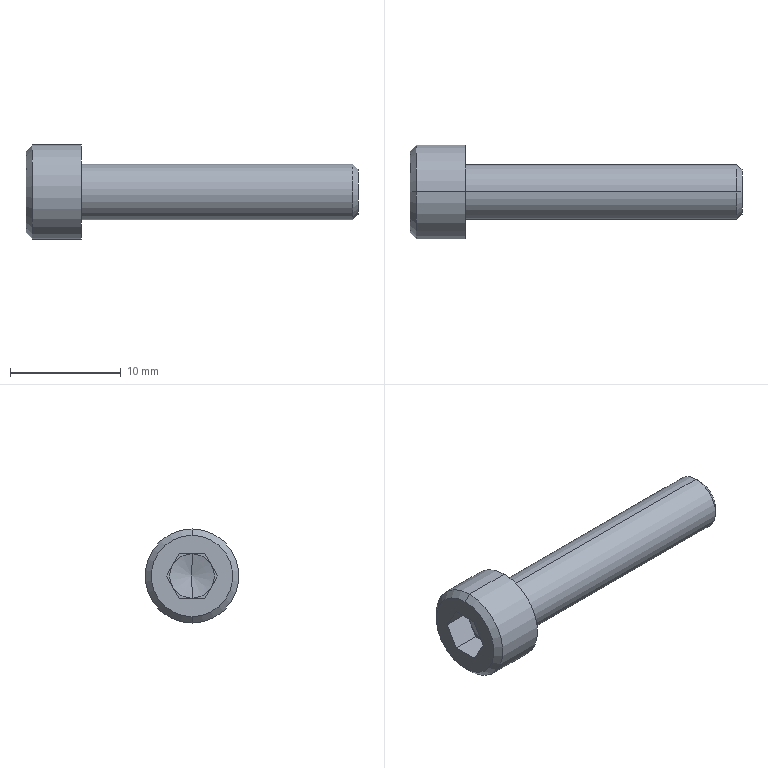Part | STEP file | CBAL5-25 | 1 solid | 25 faces | box 30 x 8.5 x 8.5 mm | volume 731.85 mm3 | plane 15 | cone 6 | cylinder 4 | commonest cylinder face diameters 5 x2 8.5 x2